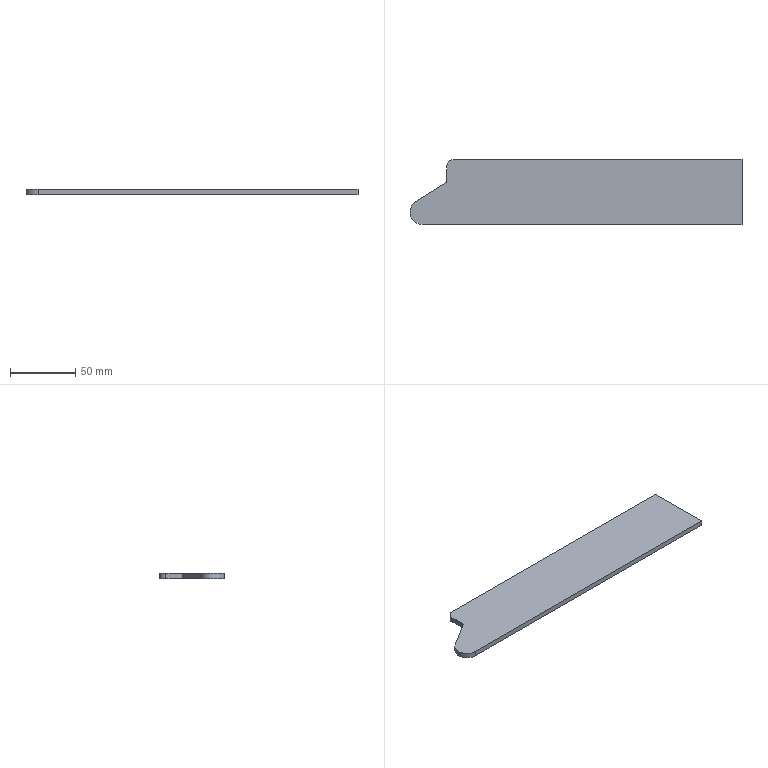Part | SolidWorks | features FlatPattern 1, SMBaseFlange 1, SheetMetal 1 | 1 solid | 9 faces | box 255 x 50 x 4 mm | volume 47889 mm3 | plane 7 | cylinder 2 | commonest cylinder face diameters 10 x1 19 x1
STEP:
#1=CARTESIAN_POINT('',(-229.485,44.403,0.));
#2=VERTEX_POINT('',#1);
#3=CARTESIAN_POINT('',(-224.452,26.846,0.));
#4=VERTEX_POINT('',#3);
#5=CARTESIAN_POINT('',(-224.452,36.346,0.));
#6=DIRECTION('',(0.,0.,1.));
#7=DIRECTION('',(1.,0.,0.));
#8=AXIS2_PLACEMENT_3D('',#5,#6,#7);
#9=CIRCLE('',#8,9.5);
#10=EDGE_CURVE('',#2,#4,#9,.T.);
#11=ORIENTED_EDGE('',*,*,#10,.F.);
#12=CARTESIAN_POINT('',(-229.485,44.403,-4.));
#13=VERTEX_POINT('',#12);
#14=CARTESIAN_POINT('',(-229.485,44.403,-4.));
#15=DIRECTION('',(0.,0.,1.));
#16=VECTOR('',#15,1000.);
#17=LINE('',#14,#16);
#18=EDGE_CURVE('',#13,#2,#17,.T.);
#19=ORIENTED_EDGE('',*,*,#18,.F.);
#20=CARTESIAN_POINT('',(-224.452,26.846,-4.));
#21=VERTEX_POINT('',#20);
#22=CARTESIAN_POINT('',(-224.452,36.346,-4.));
#23=DIRECTION('',(0.,0.,1.));
#24=DIRECTION('',(1.,0.,0.));
#25=AXIS2_PLACEMENT_3D('',#22,#23,#24);
#26=CIRCLE('',#25,9.5);
#27=EDGE_CURVE('',#13,#21,#26,.T.);
#28=ORIENTED_EDGE('',*,*,#27,.T.);
#29=CARTESIAN_POINT('',(-224.452,26.846,-4.));
#30=DIRECTION('',(0.,0.,1.));
#31=VECTOR('',#30,1000.);
#32=LINE('',#29,#31);
#33=EDGE_CURVE('',#21,#4,#32,.T.);
#34=ORIENTED_EDGE('',*,*,#33,.T.);
#35=EDGE_LOOP('',(#11,#19,#28,#34));
#36=FACE_OUTER_BOUND('',#35,.T.);
#37=CARTESIAN_POINT('',(-224.452,36.346,-4.));
#38=DIRECTION('',(0.,0.,1.));
#39=DIRECTION('',(1.,0.,0.));
#40=AXIS2_PLACEMENT_3D('',#37,#38,#39);
#41=CYLINDRICAL_SURFACE('',#40,9.5);
#42=ADVANCED_FACE('',(#36),#41,.T.);
#43=CARTESIAN_POINT('',(-205.562,59.346,0.));
#44=VERTEX_POINT('',#43);
#45=CARTESIAN_POINT('',(-205.562,59.346,0.));
#46=DIRECTION('',(-0.8481,-0.5298,0.));
#47=VECTOR('',#46,1000.);
#48=LINE('',#45,#47);
#49=EDGE_CURVE('',#44,#2,#48,.T.);
#50=ORIENTED_EDGE('',*,*,#49,.F.);
#51=CARTESIAN_POINT('',(-205.562,59.346,-4.));
#52=VERTEX_POINT('',#51);
#53=CARTESIAN_POINT('',(-205.562,59.346,-4.));
#54=DIRECTION('',(0.,0.,1.));
#55=VECTOR('',#54,1000.);
#56=LINE('',#53,#55);
#57=EDGE_CURVE('',#52,#44,#56,.T.);
#58=ORIENTED_EDGE('',*,*,#57,.F.);
#59=CARTESIAN_POINT('',(-205.562,59.346,-4.));
#60=DIRECTION('',(-0.8481,-0.5298,0.));
#61=VECTOR('',#60,1000.);
#62=LINE('',#59,#61);
#63=EDGE_CURVE('',#52,#13,#62,.T.);
#64=ORIENTED_EDGE('',*,*,#63,.T.);
#65=ORIENTED_EDGE('',*,*,#18,.T.);
#66=EDGE_LOOP('',(#50,#58,#64,#65));
#67=FACE_OUTER_BOUND('',#66,.T.);
#68=CARTESIAN_POINT('',(-205.562,59.346,-4.));
#69=DIRECTION('',(-0.5298,0.8481,0.));
#70=DIRECTION('',(-0.8481,-0.5298,0.));
#71=AXIS2_PLACEMENT_3D('',#68,#69,#70);
#72=PLANE('',#71);
#73=ADVANCED_FACE('',(#67),#72,.T.);
#74=CARTESIAN_POINT('',(-205.562,71.846,0.));
#75=VERTEX_POINT('',#74);
#76=CARTESIAN_POINT('',(-205.562,59.346,0.));
#77=DIRECTION('',(0.,-1.,0.));
#78=VECTOR('',#77,1000.);
#79=LINE('',#76,#78);
#80=EDGE_CURVE('',#75,#44,#79,.T.);
#81=ORIENTED_EDGE('',*,*,#80,.F.);
#82=CARTESIAN_POINT('',(-205.562,71.846,-4.));
#83=VERTEX_POINT('',#82);
#84=CARTESIAN_POINT('',(-205.562,71.846,-4.));
#85=DIRECTION('',(0.,0.,1.));
#86=VECTOR('',#85,1000.);
#87=LINE('',#84,#86);
#88=EDGE_CURVE('',#83,#75,#87,.T.);
#89=ORIENTED_EDGE('',*,*,#88,.F.);
#90=CARTESIAN_POINT('',(-205.562,59.346,-4.));
#91=DIRECTION('',(0.,-1.,0.));
#92=VECTOR('',#91,1000.);
#93=LINE('',#90,#92);
#94=EDGE_CURVE('',#83,#52,#93,.T.);
#95=ORIENTED_EDGE('',*,*,#94,.T.);
#96=ORIENTED_EDGE('',*,*,#57,.T.);
#97=EDGE_LOOP('',(#81,#89,#95,#96));
#98=FACE_OUTER_BOUND('',#97,.T.);
#99=CARTESIAN_POINT('',(-205.562,59.346,-4.));
#100=DIRECTION('',(-1.,0.,0.));
#101=DIRECTION('',(0.,0.,1.));
#102=AXIS2_PLACEMENT_3D('',#99,#100,#101);
#103=PLANE('',#102);
#104=ADVANCED_FACE('',(#98),#103,.T.);
#105=CARTESIAN_POINT('',(-200.562,76.846,0.));
#106=VERTEX_POINT('',#105);
#107=CARTESIAN_POINT('',(-200.562,71.846,0.));
#108=DIRECTION('',(0.,0.,1.));
#109=DIRECTION('',(1.,0.,0.));
#110=AXIS2_PLACEMENT_3D('',#107,#108,#109);
#111=CIRCLE('',#110,5.);
#112=EDGE_CURVE('',#106,#75,#111,.T.);
#113=ORIENTED_EDGE('',*,*,#112,.F.);
#114=CARTESIAN_POINT('',(-200.562,76.846,-4.));
#115=VERTEX_POINT('',#114);
#116=CARTESIAN_POINT('',(-200.562,76.846,-4.));
#117=DIRECTION('',(0.,0.,1.));
#118=VECTOR('',#117,1000.);
#119=LINE('',#116,#118);
#120=EDGE_CURVE('',#115,#106,#119,.T.);
#121=ORIENTED_EDGE('',*,*,#120,.F.);
#122=CARTESIAN_POINT('',(-200.562,71.846,-4.));
#123=DIRECTION('',(0.,0.,1.));
#124=DIRECTION('',(1.,0.,0.));
#125=AXIS2_PLACEMENT_3D('',#122,#123,#124);
#126=CIRCLE('',#125,5.);
#127=EDGE_CURVE('',#115,#83,#126,.T.);
#128=ORIENTED_EDGE('',*,*,#127,.T.);
#129=ORIENTED_EDGE('',*,*,#88,.T.);
#130=EDGE_LOOP('',(#113,#121,#128,#129));
#131=FACE_OUTER_BOUND('',#130,.T.);
#132=CARTESIAN_POINT('',(-200.562,71.846,-4.));
#133=DIRECTION('',(0.,0.,1.));
#134=DIRECTION('',(1.,0.,0.));
#135=AXIS2_PLACEMENT_3D('',#132,#133,#134);
#136=CYLINDRICAL_SURFACE('',#135,5.);
#137=ADVANCED_FACE('',(#131),#136,.T.);
#138=CARTESIAN_POINT('',(21.048,76.846,0.));
#139=VERTEX_POINT('',#138);
#140=CARTESIAN_POINT('',(-200.562,76.846,0.));
#141=DIRECTION('',(-1.,0.,0.));
#142=VECTOR('',#141,1000.);
#143=LINE('',#140,#142);
#144=EDGE_CURVE('',#139,#106,#143,.T.);
#145=ORIENTED_EDGE('',*,*,#144,.F.);
#146=CARTESIAN_POINT('',(21.048,76.846,-4.));
#147=VERTEX_POINT('',#146);
#148=CARTESIAN_POINT('',(21.048,76.846,-4.));
#149=DIRECTION('',(0.,0.,1.));
#150=VECTOR('',#149,1000.);
#151=LINE('',#148,#150);
#152=EDGE_CURVE('',#147,#139,#151,.T.);
#153=ORIENTED_EDGE('',*,*,#152,.F.);
#154=CARTESIAN_POINT('',(-200.562,76.846,-4.));
#155=DIRECTION('',(-1.,0.,0.));
#156=VECTOR('',#155,1000.);
#157=LINE('',#154,#156);
#158=EDGE_CURVE('',#147,#115,#157,.T.);
#159=ORIENTED_EDGE('',*,*,#158,.T.);
#160=ORIENTED_EDGE('',*,*,#120,.T.);
#161=EDGE_LOOP('',(#145,#153,#159,#160));
#162=FACE_OUTER_BOUND('',#161,.T.);
#163=CARTESIAN_POINT('',(-200.562,76.846,-4.));
#164=DIRECTION('',(0.,1.,0.));
#165=DIRECTION('',(-1.,0.,0.));
#166=AXIS2_PLACEMENT_3D('',#163,#164,#165);
#167=PLANE('',#166);
#168=ADVANCED_FACE('',(#162),#167,.T.);
#169=CARTESIAN_POINT('',(21.048,26.846,0.));
#170=VERTEX_POINT('',#169);
#171=CARTESIAN_POINT('',(21.048,26.846,0.));
#172=DIRECTION('',(0.,1.,0.));
#173=VECTOR('',#172,1000.);
#174=LINE('',#171,#173);
#175=EDGE_CURVE('',#170,#139,#174,.T.);
#176=ORIENTED_EDGE('',*,*,#175,.F.);
#177=CARTESIAN_POINT('',(21.048,26.846,-4.));
#178=VERTEX_POINT('',#177);
#179=CARTESIAN_POINT('',(21.048,26.846,-4.));
#180=DIRECTION('',(0.,0.,1.));
#181=VECTOR('',#180,1000.);
#182=LINE('',#179,#181);
#183=EDGE_CURVE('',#178,#170,#182,.T.);
#184=ORIENTED_EDGE('',*,*,#183,.F.);
#185=CARTESIAN_POINT('',(21.048,26.846,-4.));
#186=DIRECTION('',(0.,1.,0.));
#187=VECTOR('',#186,1000.);
#188=LINE('',#185,#187);
#189=EDGE_CURVE('',#178,#147,#188,.T.);
#190=ORIENTED_EDGE('',*,*,#189,.T.);
#191=ORIENTED_EDGE('',*,*,#152,.T.);
#192=EDGE_LOOP('',(#176,#184,#190,#191));
#193=FACE_OUTER_BOUND('',#192,.T.);
#194=CARTESIAN_POINT('',(21.048,26.846,-4.));
#195=DIRECTION('',(1.,0.,0.));
#196=DIRECTION('',(0.,0.,-1.));
#197=AXIS2_PLACEMENT_3D('',#194,#195,#196);
#198=PLANE('',#197);
#199=ADVANCED_FACE('',(#193),#198,.T.);
#200=CARTESIAN_POINT('',(-224.452,26.846,0.));
#201=DIRECTION('',(1.,0.,0.));
#202=VECTOR('',#201,1000.);
#203=LINE('',#200,#202);
#204=EDGE_CURVE('',#4,#170,#203,.T.);
#205=ORIENTED_EDGE('',*,*,#204,.F.);
#206=ORIENTED_EDGE('',*,*,#33,.F.);
#207=CARTESIAN_POINT('',(-224.452,26.846,-4.));
#208=DIRECTION('',(1.,0.,0.));
#209=VECTOR('',#208,1000.);
#210=LINE('',#207,#209);
#211=EDGE_CURVE('',#21,#178,#210,.T.);
#212=ORIENTED_EDGE('',*,*,#211,.T.);
#213=ORIENTED_EDGE('',*,*,#183,.T.);
#214=EDGE_LOOP('',(#205,#206,#212,#213));
#215=FACE_OUTER_BOUND('',#214,.T.);
#216=CARTESIAN_POINT('',(-224.452,26.846,-4.));
#217=DIRECTION('',(0.,-1.,0.));
#218=DIRECTION('',(1.,0.,0.));
#219=AXIS2_PLACEMENT_3D('',#216,#217,#218);
#220=PLANE('',#219);
#221=ADVANCED_FACE('',(#215),#220,.T.);
#222=ORIENTED_EDGE('',*,*,#27,.F.);
#223=ORIENTED_EDGE('',*,*,#63,.F.);
#224=ORIENTED_EDGE('',*,*,#94,.F.);
#225=ORIENTED_EDGE('',*,*,#127,.F.);
#226=ORIENTED_EDGE('',*,*,#158,.F.);
#227=ORIENTED_EDGE('',*,*,#189,.F.);
#228=ORIENTED_EDGE('',*,*,#211,.F.);
#229=EDGE_LOOP('',(#222,#223,#224,#225,#226,#227,#228));
#230=FACE_OUTER_BOUND('',#229,.T.);
#231=CARTESIAN_POINT('',(-224.452,36.346,-4.));
#232=DIRECTION('',(0.,0.,1.));
#233=DIRECTION('',(1.,0.,0.));
#234=AXIS2_PLACEMENT_3D('',#231,#232,#233);
#235=PLANE('',#234);
#236=ADVANCED_FACE('',(#230),#235,.F.);
#237=ORIENTED_EDGE('',*,*,#10,.T.);
#238=ORIENTED_EDGE('',*,*,#204,.T.);
#239=ORIENTED_EDGE('',*,*,#175,.T.);
#240=ORIENTED_EDGE('',*,*,#144,.T.);
#241=ORIENTED_EDGE('',*,*,#112,.T.);
#242=ORIENTED_EDGE('',*,*,#80,.T.);
#243=ORIENTED_EDGE('',*,*,#49,.T.);
#244=EDGE_LOOP('',(#237,#238,#239,#240,#241,#242,#243));
#245=FACE_OUTER_BOUND('',#244,.T.);
#246=CARTESIAN_POINT('',(-224.452,36.346,0.));
#247=DIRECTION('',(0.,0.,1.));
#248=DIRECTION('',(1.,0.,0.));
#249=AXIS2_PLACEMENT_3D('',#246,#247,#248);
#250=PLANE('',#249);
#251=ADVANCED_FACE('',(#245),#250,.T.);
#252=CLOSED_SHELL('',(#42,#73,#104,#137,#168,#199,#221,#236,#251));
#253=MANIFOLD_SOLID_BREP('',#252);
#254=CARTESIAN_POINT('',(0.,0.,0.));
#255=DIRECTION('',(0.,0.,1.));
#256=DIRECTION('',(1.,0.,0.));
#257=AXIS2_PLACEMENT_3D('',#254,#255,#256);
#258=(LENGTH_UNIT()NAMED_UNIT(*)SI_UNIT(.MILLI.,.METRE.));
#259=UNCERTAINTY_MEASURE_WITH_UNIT(LENGTH_MEASURE(0.00001),#258,'','');
#260=(NAMED_UNIT(*)PLANE_ANGLE_UNIT()SI_UNIT($,.RADIAN.));
#261=(NAMED_UNIT(*)SI_UNIT($,.STERADIAN.)SOLID_ANGLE_UNIT());
#262=(GEOMETRIC_REPRESENTATION_CONTEXT(3)GLOBAL_UNCERTAINTY_ASSIGNED_CONTEXT((#259))GLOBAL_UNIT_ASSIGNED_CONTEXT((#258,#260,#261))REPRESENTATION_CONTEXT('',''));
#263=ADVANCED_BREP_SHAPE_REPRESENTATION('',(#253,#257),#262);